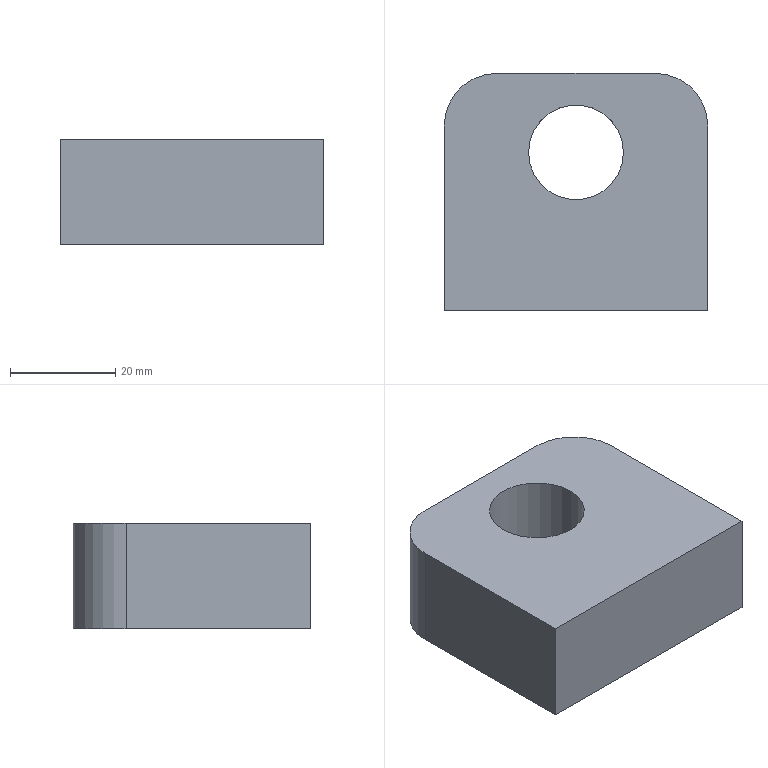Part | SolidWorks | features Extrusion 1, Fillet 1 | 1 solid | 10 faces | box 50 x 45 x 20 mm | volume 39052 mm3 | plane 6 | cylinder 4 | commonest cylinder face diameters 18 x2 20 x2
STEP:
#1=CARTESIAN_POINT('',(16.,30.,20.));
#2=VERTEX_POINT('',#1);
#3=CARTESIAN_POINT('',(34.,30.,20.));
#4=VERTEX_POINT('',#3);
#5=CARTESIAN_POINT('',(25.,30.,20.));
#6=DIRECTION('',(0.,0.,1.));
#7=DIRECTION('',(1.,0.,0.));
#8=AXIS2_PLACEMENT_3D('',#5,#6,#7);
#9=CIRCLE('',#8,9.);
#10=EDGE_CURVE('',#2,#4,#9,.T.);
#11=ORIENTED_EDGE('',*,*,#10,.T.);
#12=CARTESIAN_POINT('',(34.,30.,0.));
#13=VERTEX_POINT('',#12);
#14=CARTESIAN_POINT('',(34.,30.,20.));
#15=DIRECTION('',(0.,0.,-1.));
#16=VECTOR('',#15,1000.);
#17=LINE('',#14,#16);
#18=EDGE_CURVE('',#4,#13,#17,.T.);
#19=ORIENTED_EDGE('',*,*,#18,.T.);
#20=CARTESIAN_POINT('',(16.,30.,0.));
#21=VERTEX_POINT('',#20);
#22=CARTESIAN_POINT('',(25.,30.,0.));
#23=DIRECTION('',(0.,0.,1.));
#24=DIRECTION('',(1.,0.,0.));
#25=AXIS2_PLACEMENT_3D('',#22,#23,#24);
#26=CIRCLE('',#25,9.);
#27=EDGE_CURVE('',#21,#13,#26,.T.);
#28=ORIENTED_EDGE('',*,*,#27,.F.);
#29=CARTESIAN_POINT('',(16.,30.,20.));
#30=DIRECTION('',(0.,0.,-1.));
#31=VECTOR('',#30,1000.);
#32=LINE('',#29,#31);
#33=EDGE_CURVE('',#2,#21,#32,.T.);
#34=ORIENTED_EDGE('',*,*,#33,.F.);
#35=EDGE_LOOP('',(#11,#19,#28,#34));
#36=FACE_OUTER_BOUND('',#35,.T.);
#37=CARTESIAN_POINT('',(25.,30.,20.));
#38=DIRECTION('',(0.,0.,-1.));
#39=DIRECTION('',(-1.,0.,0.));
#40=AXIS2_PLACEMENT_3D('',#37,#38,#39);
#41=CYLINDRICAL_SURFACE('',#40,9.);
#42=ADVANCED_FACE('',(#36),#41,.F.);
#43=CARTESIAN_POINT('',(40.,45.,20.));
#44=VERTEX_POINT('',#43);
#45=CARTESIAN_POINT('',(10.,45.,20.));
#46=VERTEX_POINT('',#45);
#47=CARTESIAN_POINT('',(0.,45.,20.));
#48=DIRECTION('',(-1.,0.,0.));
#49=VECTOR('',#48,1000.);
#50=LINE('',#47,#49);
#51=EDGE_CURVE('',#44,#46,#50,.T.);
#52=ORIENTED_EDGE('',*,*,#51,.T.);
#53=CARTESIAN_POINT('',(0.,35.,20.));
#54=VERTEX_POINT('',#53);
#55=CARTESIAN_POINT('',(10.,35.,20.));
#56=DIRECTION('',(0.,0.,1.));
#57=DIRECTION('',(-1.,0.,0.));
#58=AXIS2_PLACEMENT_3D('',#55,#56,#57);
#59=CIRCLE('',#58,10.);
#60=EDGE_CURVE('',#46,#54,#59,.T.);
#61=ORIENTED_EDGE('',*,*,#60,.T.);
#62=CARTESIAN_POINT('',(0.,0.,20.));
#63=VERTEX_POINT('',#62);
#64=CARTESIAN_POINT('',(0.,0.,20.));
#65=DIRECTION('',(0.,-1.,0.));
#66=VECTOR('',#65,1000.);
#67=LINE('',#64,#66);
#68=EDGE_CURVE('',#54,#63,#67,.T.);
#69=ORIENTED_EDGE('',*,*,#68,.T.);
#70=CARTESIAN_POINT('',(50.,0.,20.));
#71=VERTEX_POINT('',#70);
#72=CARTESIAN_POINT('',(0.,0.,20.));
#73=DIRECTION('',(1.,0.,0.));
#74=VECTOR('',#73,1000.);
#75=LINE('',#72,#74);
#76=EDGE_CURVE('',#63,#71,#75,.T.);
#77=ORIENTED_EDGE('',*,*,#76,.T.);
#78=CARTESIAN_POINT('',(50.,35.,20.));
#79=VERTEX_POINT('',#78);
#80=CARTESIAN_POINT('',(50.,0.,20.));
#81=DIRECTION('',(0.,1.,0.));
#82=VECTOR('',#81,1000.);
#83=LINE('',#80,#82);
#84=EDGE_CURVE('',#71,#79,#83,.T.);
#85=ORIENTED_EDGE('',*,*,#84,.T.);
#86=CARTESIAN_POINT('',(40.,35.,20.));
#87=DIRECTION('',(0.,0.,1.));
#88=DIRECTION('',(-1.,0.,0.));
#89=AXIS2_PLACEMENT_3D('',#86,#87,#88);
#90=CIRCLE('',#89,10.);
#91=EDGE_CURVE('',#79,#44,#90,.T.);
#92=ORIENTED_EDGE('',*,*,#91,.T.);
#93=EDGE_LOOP('',(#52,#61,#69,#77,#85,#92));
#94=FACE_OUTER_BOUND('',#93,.T.);
#95=ORIENTED_EDGE('',*,*,#10,.F.);
#96=CARTESIAN_POINT('',(25.,30.,20.));
#97=DIRECTION('',(0.,0.,1.));
#98=DIRECTION('',(1.,0.,0.));
#99=AXIS2_PLACEMENT_3D('',#96,#97,#98);
#100=CIRCLE('',#99,9.);
#101=EDGE_CURVE('',#4,#2,#100,.T.);
#102=ORIENTED_EDGE('',*,*,#101,.F.);
#103=EDGE_LOOP('',(#95,#102));
#104=FACE_BOUND('',#103,.T.);
#105=CARTESIAN_POINT('',(0.,0.,20.));
#106=DIRECTION('',(0.,0.,-1.));
#107=DIRECTION('',(-1.,0.,0.));
#108=AXIS2_PLACEMENT_3D('',#105,#106,#107);
#109=PLANE('',#108);
#110=ADVANCED_FACE('',(#94,#104),#109,.F.);
#111=CARTESIAN_POINT('',(0.,35.,0.));
#112=VERTEX_POINT('',#111);
#113=CARTESIAN_POINT('',(0.,0.,0.));
#114=VERTEX_POINT('',#113);
#115=CARTESIAN_POINT('',(0.,0.,0.));
#116=DIRECTION('',(0.,-1.,0.));
#117=VECTOR('',#116,1000.);
#118=LINE('',#115,#117);
#119=EDGE_CURVE('',#112,#114,#118,.T.);
#120=ORIENTED_EDGE('',*,*,#119,.F.);
#121=CARTESIAN_POINT('',(10.,45.,0.));
#122=VERTEX_POINT('',#121);
#123=CARTESIAN_POINT('',(10.,35.,0.));
#124=DIRECTION('',(0.,0.,-1.));
#125=DIRECTION('',(-1.,0.,0.));
#126=AXIS2_PLACEMENT_3D('',#123,#124,#125);
#127=CIRCLE('',#126,10.);
#128=EDGE_CURVE('',#112,#122,#127,.T.);
#129=ORIENTED_EDGE('',*,*,#128,.T.);
#130=CARTESIAN_POINT('',(40.,45.,0.));
#131=VERTEX_POINT('',#130);
#132=CARTESIAN_POINT('',(0.,45.,0.));
#133=DIRECTION('',(-1.,0.,0.));
#134=VECTOR('',#133,1000.);
#135=LINE('',#132,#134);
#136=EDGE_CURVE('',#131,#122,#135,.T.);
#137=ORIENTED_EDGE('',*,*,#136,.F.);
#138=CARTESIAN_POINT('',(50.,35.,0.));
#139=VERTEX_POINT('',#138);
#140=CARTESIAN_POINT('',(40.,35.,0.));
#141=DIRECTION('',(0.,0.,-1.));
#142=DIRECTION('',(-1.,0.,0.));
#143=AXIS2_PLACEMENT_3D('',#140,#141,#142);
#144=CIRCLE('',#143,10.);
#145=EDGE_CURVE('',#131,#139,#144,.T.);
#146=ORIENTED_EDGE('',*,*,#145,.T.);
#147=CARTESIAN_POINT('',(50.,0.,0.));
#148=VERTEX_POINT('',#147);
#149=CARTESIAN_POINT('',(50.,0.,0.));
#150=DIRECTION('',(0.,1.,0.));
#151=VECTOR('',#150,1000.);
#152=LINE('',#149,#151);
#153=EDGE_CURVE('',#148,#139,#152,.T.);
#154=ORIENTED_EDGE('',*,*,#153,.F.);
#155=CARTESIAN_POINT('',(0.,0.,0.));
#156=DIRECTION('',(1.,0.,0.));
#157=VECTOR('',#156,1000.);
#158=LINE('',#155,#157);
#159=EDGE_CURVE('',#114,#148,#158,.T.);
#160=ORIENTED_EDGE('',*,*,#159,.F.);
#161=EDGE_LOOP('',(#120,#129,#137,#146,#154,#160));
#162=FACE_OUTER_BOUND('',#161,.T.);
#163=ORIENTED_EDGE('',*,*,#27,.T.);
#164=CARTESIAN_POINT('',(25.,30.,0.));
#165=DIRECTION('',(0.,0.,1.));
#166=DIRECTION('',(1.,0.,0.));
#167=AXIS2_PLACEMENT_3D('',#164,#165,#166);
#168=CIRCLE('',#167,9.);
#169=EDGE_CURVE('',#13,#21,#168,.T.);
#170=ORIENTED_EDGE('',*,*,#169,.T.);
#171=EDGE_LOOP('',(#163,#170));
#172=FACE_BOUND('',#171,.T.);
#173=CARTESIAN_POINT('',(0.,0.,0.));
#174=DIRECTION('',(0.,0.,-1.));
#175=DIRECTION('',(-1.,0.,0.));
#176=AXIS2_PLACEMENT_3D('',#173,#174,#175);
#177=PLANE('',#176);
#178=ADVANCED_FACE('',(#162,#172),#177,.T.);
#179=ORIENTED_EDGE('',*,*,#68,.F.);
#180=CARTESIAN_POINT('',(0.,35.,20.));
#181=DIRECTION('',(0.,0.,-1.));
#182=VECTOR('',#181,1000.);
#183=LINE('',#180,#182);
#184=EDGE_CURVE('',#54,#112,#183,.T.);
#185=ORIENTED_EDGE('',*,*,#184,.T.);
#186=ORIENTED_EDGE('',*,*,#119,.T.);
#187=CARTESIAN_POINT('',(0.,0.,20.));
#188=DIRECTION('',(0.,0.,-1.));
#189=VECTOR('',#188,1000.);
#190=LINE('',#187,#189);
#191=EDGE_CURVE('',#63,#114,#190,.T.);
#192=ORIENTED_EDGE('',*,*,#191,.F.);
#193=EDGE_LOOP('',(#179,#185,#186,#192));
#194=FACE_OUTER_BOUND('',#193,.T.);
#195=CARTESIAN_POINT('',(0.,0.,20.));
#196=DIRECTION('',(1.,0.,0.));
#197=DIRECTION('',(0.,0.,-1.));
#198=AXIS2_PLACEMENT_3D('',#195,#196,#197);
#199=PLANE('',#198);
#200=ADVANCED_FACE('',(#194),#199,.F.);
#201=ORIENTED_EDGE('',*,*,#159,.T.);
#202=CARTESIAN_POINT('',(50.,0.,20.));
#203=DIRECTION('',(0.,0.,-1.));
#204=VECTOR('',#203,1000.);
#205=LINE('',#202,#204);
#206=EDGE_CURVE('',#71,#148,#205,.T.);
#207=ORIENTED_EDGE('',*,*,#206,.F.);
#208=ORIENTED_EDGE('',*,*,#76,.F.);
#209=ORIENTED_EDGE('',*,*,#191,.T.);
#210=EDGE_LOOP('',(#201,#207,#208,#209));
#211=FACE_OUTER_BOUND('',#210,.T.);
#212=CARTESIAN_POINT('',(0.,0.,20.));
#213=DIRECTION('',(0.,1.,0.));
#214=DIRECTION('',(0.,0.,1.));
#215=AXIS2_PLACEMENT_3D('',#212,#213,#214);
#216=PLANE('',#215);
#217=ADVANCED_FACE('',(#211),#216,.F.);
#218=ORIENTED_EDGE('',*,*,#153,.T.);
#219=CARTESIAN_POINT('',(50.,35.,20.));
#220=DIRECTION('',(0.,0.,1.));
#221=VECTOR('',#220,1000.);
#222=LINE('',#219,#221);
#223=EDGE_CURVE('',#139,#79,#222,.T.);
#224=ORIENTED_EDGE('',*,*,#223,.T.);
#225=ORIENTED_EDGE('',*,*,#84,.F.);
#226=ORIENTED_EDGE('',*,*,#206,.T.);
#227=EDGE_LOOP('',(#218,#224,#225,#226));
#228=FACE_OUTER_BOUND('',#227,.T.);
#229=CARTESIAN_POINT('',(50.,0.,20.));
#230=DIRECTION('',(-1.,0.,0.));
#231=DIRECTION('',(0.,0.,1.));
#232=AXIS2_PLACEMENT_3D('',#229,#230,#231);
#233=PLANE('',#232);
#234=ADVANCED_FACE('',(#228),#233,.F.);
#235=ORIENTED_EDGE('',*,*,#136,.T.);
#236=CARTESIAN_POINT('',(10.,45.,20.));
#237=DIRECTION('',(0.,0.,1.));
#238=VECTOR('',#237,1000.);
#239=LINE('',#236,#238);
#240=EDGE_CURVE('',#122,#46,#239,.T.);
#241=ORIENTED_EDGE('',*,*,#240,.T.);
#242=ORIENTED_EDGE('',*,*,#51,.F.);
#243=CARTESIAN_POINT('',(40.,45.,20.));
#244=DIRECTION('',(0.,0.,-1.));
#245=VECTOR('',#244,1000.);
#246=LINE('',#243,#245);
#247=EDGE_CURVE('',#44,#131,#246,.T.);
#248=ORIENTED_EDGE('',*,*,#247,.T.);
#249=EDGE_LOOP('',(#235,#241,#242,#248));
#250=FACE_OUTER_BOUND('',#249,.T.);
#251=CARTESIAN_POINT('',(0.,45.,20.));
#252=DIRECTION('',(0.,-1.,0.));
#253=DIRECTION('',(0.,0.,-1.));
#254=AXIS2_PLACEMENT_3D('',#251,#252,#253);
#255=PLANE('',#254);
#256=ADVANCED_FACE('',(#250),#255,.F.);
#257=ORIENTED_EDGE('',*,*,#18,.F.);
#258=ORIENTED_EDGE('',*,*,#101,.T.);
#259=ORIENTED_EDGE('',*,*,#33,.T.);
#260=ORIENTED_EDGE('',*,*,#169,.F.);
#261=EDGE_LOOP('',(#257,#258,#259,#260));
#262=FACE_OUTER_BOUND('',#261,.T.);
#263=CARTESIAN_POINT('',(25.,30.,20.));
#264=DIRECTION('',(0.,0.,-1.));
#265=DIRECTION('',(-1.,0.,0.));
#266=AXIS2_PLACEMENT_3D('',#263,#264,#265);
#267=CYLINDRICAL_SURFACE('',#266,9.);
#268=ADVANCED_FACE('',(#262),#267,.F.);
#269=ORIENTED_EDGE('',*,*,#60,.F.);
#270=ORIENTED_EDGE('',*,*,#240,.F.);
#271=ORIENTED_EDGE('',*,*,#128,.F.);
#272=ORIENTED_EDGE('',*,*,#184,.F.);
#273=EDGE_LOOP('',(#269,#270,#271,#272));
#274=FACE_OUTER_BOUND('',#273,.T.);
#275=CARTESIAN_POINT('',(10.,35.,20.));
#276=DIRECTION('',(0.,0.,-1.));
#277=DIRECTION('',(-1.,0.,0.));
#278=AXIS2_PLACEMENT_3D('',#275,#276,#277);
#279=CYLINDRICAL_SURFACE('',#278,10.);
#280=ADVANCED_FACE('',(#274),#279,.T.);
#281=ORIENTED_EDGE('',*,*,#91,.F.);
#282=ORIENTED_EDGE('',*,*,#223,.F.);
#283=ORIENTED_EDGE('',*,*,#145,.F.);
#284=ORIENTED_EDGE('',*,*,#247,.F.);
#285=EDGE_LOOP('',(#281,#282,#283,#284));
#286=FACE_OUTER_BOUND('',#285,.T.);
#287=CARTESIAN_POINT('',(40.,35.,20.));
#288=DIRECTION('',(0.,0.,-1.));
#289=DIRECTION('',(-1.,0.,0.));
#290=AXIS2_PLACEMENT_3D('',#287,#288,#289);
#291=CYLINDRICAL_SURFACE('',#290,10.);
#292=ADVANCED_FACE('',(#286),#291,.T.);
#293=CLOSED_SHELL('',(#42,#110,#178,#200,#217,#234,#256,#268,#280,#292));
#294=MANIFOLD_SOLID_BREP('',#293);
#295=CARTESIAN_POINT('',(0.,0.,0.));
#296=DIRECTION('',(0.,0.,1.));
#297=DIRECTION('',(1.,0.,0.));
#298=AXIS2_PLACEMENT_3D('',#295,#296,#297);
#299=(LENGTH_UNIT()NAMED_UNIT(*)SI_UNIT(.MILLI.,.METRE.));
#300=UNCERTAINTY_MEASURE_WITH_UNIT(LENGTH_MEASURE(0.00001),#299,'','');
#301=(NAMED_UNIT(*)PLANE_ANGLE_UNIT()SI_UNIT($,.RADIAN.));
#302=(NAMED_UNIT(*)SI_UNIT($,.STERADIAN.)SOLID_ANGLE_UNIT());
#303=(GEOMETRIC_REPRESENTATION_CONTEXT(3)GLOBAL_UNCERTAINTY_ASSIGNED_CONTEXT((#300))GLOBAL_UNIT_ASSIGNED_CONTEXT((#299,#301,#302))REPRESENTATION_CONTEXT('',''));
#304=ADVANCED_BREP_SHAPE_REPRESENTATION('',(#294,#298),#303);